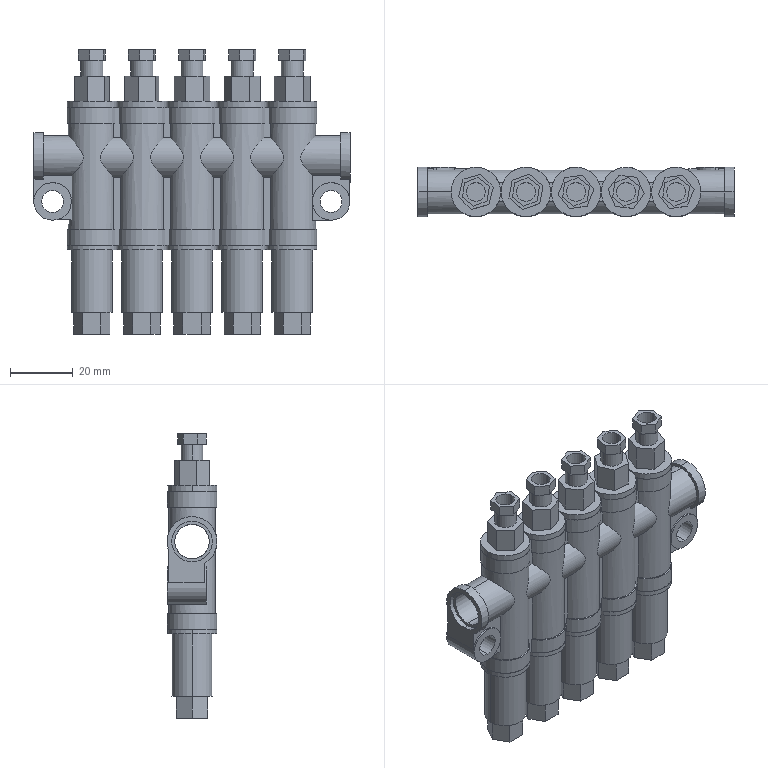Part | STEP file | 5-Way Oil Manifold | 11 solids | 407 faces | box 101.057 x 16 x 91 mm | volume 41067 mm3 | plane 242 | cylinder 165 | commonest cylinder face diameters 15.8 x38 6 x20 12.8 x18 7 x14 12 x14 13 x14